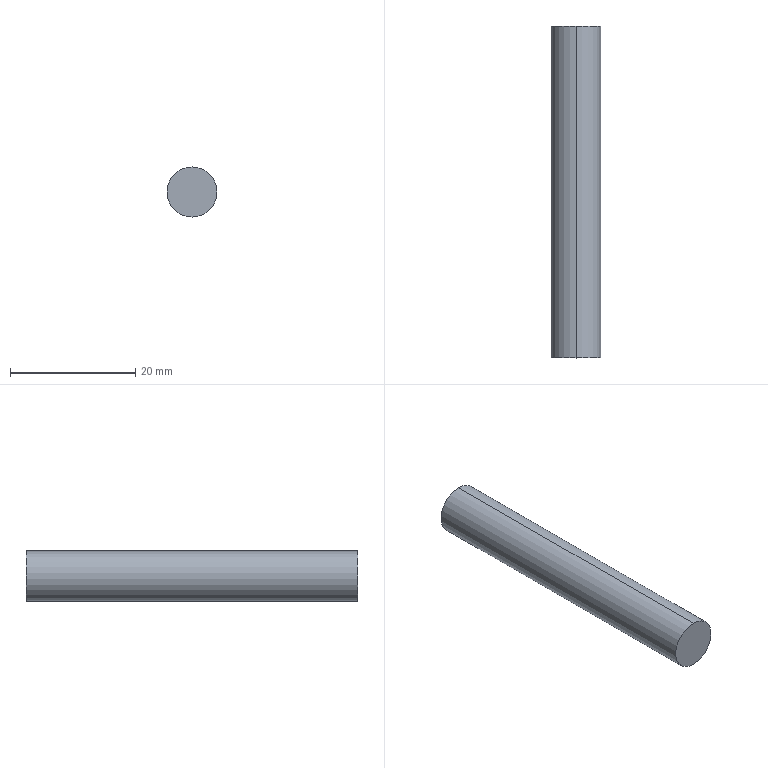Part | SolidWorks | features Extrusion 1 | 1 solid | 4 faces | box 8 x 53 x 8 mm | volume 2664 mm3 | cylinder 2 | plane 2 | commonest cylinder face diameters 8 x2
STEP:
#1=CARTESIAN_POINT('',(0.,53.,4.));
#2=VERTEX_POINT('',#1);
#3=CARTESIAN_POINT('',(0.,53.,-4.));
#4=VERTEX_POINT('',#3);
#5=CARTESIAN_POINT('',(0.,53.,0.));
#6=DIRECTION('',(0.,1.,0.));
#7=DIRECTION('',(0.,0.,1.));
#8=AXIS2_PLACEMENT_3D('',#5,#6,#7);
#9=CIRCLE('',#8,4.);
#10=EDGE_CURVE('',#2,#4,#9,.T.);
#11=ORIENTED_EDGE('',*,*,#10,.F.);
#12=CARTESIAN_POINT('',(0.,0.,4.));
#13=VERTEX_POINT('',#12);
#14=CARTESIAN_POINT('',(0.,53.,4.));
#15=DIRECTION('',(0.,-1.,0.));
#16=VECTOR('',#15,1000.);
#17=LINE('',#14,#16);
#18=EDGE_CURVE('',#2,#13,#17,.T.);
#19=ORIENTED_EDGE('',*,*,#18,.T.);
#20=CARTESIAN_POINT('',(0.,0.,-4.));
#21=VERTEX_POINT('',#20);
#22=CARTESIAN_POINT('',(0.,0.,0.));
#23=DIRECTION('',(0.,1.,0.));
#24=DIRECTION('',(0.,0.,1.));
#25=AXIS2_PLACEMENT_3D('',#22,#23,#24);
#26=CIRCLE('',#25,4.);
#27=EDGE_CURVE('',#13,#21,#26,.T.);
#28=ORIENTED_EDGE('',*,*,#27,.T.);
#29=CARTESIAN_POINT('',(0.,53.,-4.));
#30=DIRECTION('',(0.,-1.,0.));
#31=VECTOR('',#30,1000.);
#32=LINE('',#29,#31);
#33=EDGE_CURVE('',#4,#21,#32,.T.);
#34=ORIENTED_EDGE('',*,*,#33,.F.);
#35=EDGE_LOOP('',(#11,#19,#28,#34));
#36=FACE_OUTER_BOUND('',#35,.T.);
#37=CARTESIAN_POINT('',(0.,53.,0.));
#38=DIRECTION('',(0.,-1.,0.));
#39=DIRECTION('',(0.,0.,-1.));
#40=AXIS2_PLACEMENT_3D('',#37,#38,#39);
#41=CYLINDRICAL_SURFACE('',#40,4.);
#42=ADVANCED_FACE('',(#36),#41,.T.);
#43=ORIENTED_EDGE('',*,*,#18,.F.);
#44=CARTESIAN_POINT('',(0.,53.,0.));
#45=DIRECTION('',(0.,1.,0.));
#46=DIRECTION('',(0.,0.,1.));
#47=AXIS2_PLACEMENT_3D('',#44,#45,#46);
#48=CIRCLE('',#47,4.);
#49=EDGE_CURVE('',#4,#2,#48,.T.);
#50=ORIENTED_EDGE('',*,*,#49,.F.);
#51=ORIENTED_EDGE('',*,*,#33,.T.);
#52=CARTESIAN_POINT('',(0.,0.,0.));
#53=DIRECTION('',(0.,1.,0.));
#54=DIRECTION('',(0.,0.,1.));
#55=AXIS2_PLACEMENT_3D('',#52,#53,#54);
#56=CIRCLE('',#55,4.);
#57=EDGE_CURVE('',#21,#13,#56,.T.);
#58=ORIENTED_EDGE('',*,*,#57,.T.);
#59=EDGE_LOOP('',(#43,#50,#51,#58));
#60=FACE_OUTER_BOUND('',#59,.T.);
#61=CARTESIAN_POINT('',(0.,53.,0.));
#62=DIRECTION('',(0.,-1.,0.));
#63=DIRECTION('',(0.,0.,-1.));
#64=AXIS2_PLACEMENT_3D('',#61,#62,#63);
#65=CYLINDRICAL_SURFACE('',#64,4.);
#66=ADVANCED_FACE('',(#60),#65,.T.);
#67=ORIENTED_EDGE('',*,*,#49,.T.);
#68=ORIENTED_EDGE('',*,*,#10,.T.);
#69=EDGE_LOOP('',(#67,#68));
#70=FACE_OUTER_BOUND('',#69,.T.);
#71=CARTESIAN_POINT('',(0.,53.,0.));
#72=DIRECTION('',(0.,1.,0.));
#73=DIRECTION('',(0.,0.,1.));
#74=AXIS2_PLACEMENT_3D('',#71,#72,#73);
#75=PLANE('',#74);
#76=ADVANCED_FACE('',(#70),#75,.T.);
#77=ORIENTED_EDGE('',*,*,#57,.F.);
#78=ORIENTED_EDGE('',*,*,#27,.F.);
#79=EDGE_LOOP('',(#77,#78));
#80=FACE_OUTER_BOUND('',#79,.T.);
#81=CARTESIAN_POINT('',(0.,0.,0.));
#82=DIRECTION('',(0.,1.,0.));
#83=DIRECTION('',(0.,0.,1.));
#84=AXIS2_PLACEMENT_3D('',#81,#82,#83);
#85=PLANE('',#84);
#86=ADVANCED_FACE('',(#80),#85,.F.);
#87=CLOSED_SHELL('',(#42,#66,#76,#86));
#88=MANIFOLD_SOLID_BREP('',#87);
#89=CARTESIAN_POINT('',(0.,0.,0.));
#90=DIRECTION('',(0.,0.,1.));
#91=DIRECTION('',(1.,0.,0.));
#92=AXIS2_PLACEMENT_3D('',#89,#90,#91);
#93=(LENGTH_UNIT()NAMED_UNIT(*)SI_UNIT(.MILLI.,.METRE.));
#94=UNCERTAINTY_MEASURE_WITH_UNIT(LENGTH_MEASURE(0.00001),#93,'','');
#95=(NAMED_UNIT(*)PLANE_ANGLE_UNIT()SI_UNIT($,.RADIAN.));
#96=(NAMED_UNIT(*)SI_UNIT($,.STERADIAN.)SOLID_ANGLE_UNIT());
#97=(GEOMETRIC_REPRESENTATION_CONTEXT(3)GLOBAL_UNCERTAINTY_ASSIGNED_CONTEXT((#94))GLOBAL_UNIT_ASSIGNED_CONTEXT((#93,#95,#96))REPRESENTATION_CONTEXT('',''));
#98=ADVANCED_BREP_SHAPE_REPRESENTATION('',(#88,#92),#97);